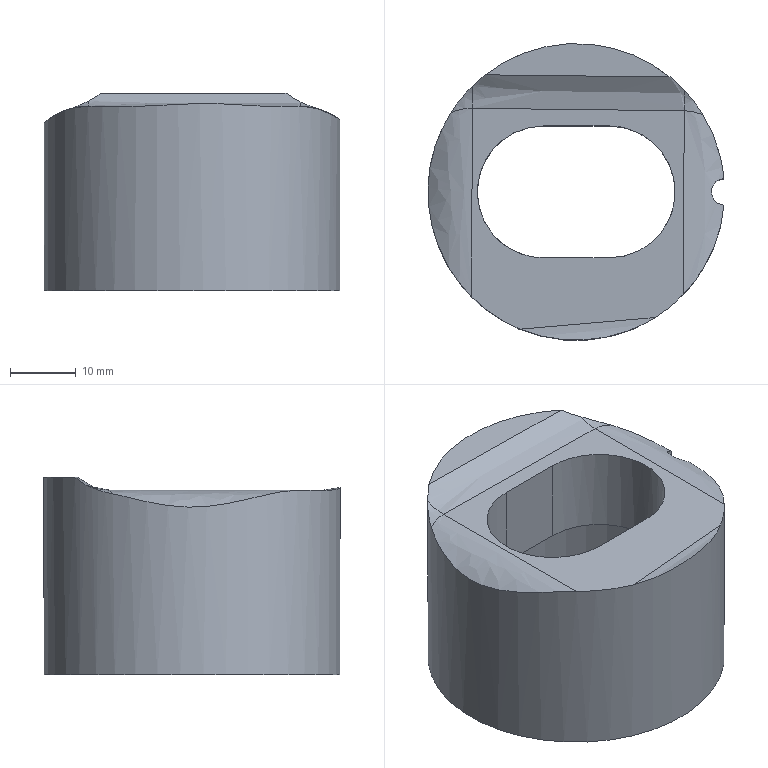Part | NX | features solid 2 | 1 solid | 17 faces | box 44.911 x 45 x 30 mm | volume 22561 mm3 | plane 6 | spline 6 | cylinder 5 | commonest cylinder face diameters 20 x2 4 x1 36 x1 45 x1
STEP:
#1=CARTESIAN_POINT('',(872.412,-199.998,17.));
#2=VERTEX_POINT('',#1);
#3=CARTESIAN_POINT('',(872.412,-199.998,42.909));
#4=VERTEX_POINT('',#3);
#5=CARTESIAN_POINT('',(872.412,-199.998,32.));
#6=DIRECTION('',(0.,0.,-1.));
#7=VECTOR('',#6,1000.);
#8=LINE('',#5,#7);
#9=EDGE_CURVE('',#2,#4,#8,.F.);
#10=ORIENTED_EDGE('',*,*,#9,.T.);
#11=CARTESIAN_POINT('',(866.197,-213.618,45.));
#12=VERTEX_POINT('',#11);
#13=CARTESIAN_POINT('',(872.412,-199.998,42.909));
#14=CARTESIAN_POINT('',(872.182,-202.576,43.073));
#15=CARTESIAN_POINT('',(870.861,-207.494,44.082));
#16=CARTESIAN_POINT('',(867.998,-211.75,45.));
#17=CARTESIAN_POINT('',(866.197,-213.618,45.));
#18=B_SPLINE_CURVE_WITH_KNOTS('',3,(#13,#14,#15,#16,#17),.UNSPECIFIED.,.F.,.F.,(4,1,4),(0.,0.007673,0.01535),.UNSPECIFIED.);
#19=EDGE_CURVE('',#4,#12,#18,.T.);
#20=ORIENTED_EDGE('',*,*,#19,.T.);
#21=CARTESIAN_POINT('',(861.953,-217.062,45.));
#22=VERTEX_POINT('',#21);
#23=CARTESIAN_POINT('',(850.,-198.,45.));
#24=DIRECTION('',(0.,0.,-1.));
#25=DIRECTION('',(-1.,0.,0.));
#26=AXIS2_PLACEMENT_3D('',#23,#24,#25);
#27=CIRCLE('',#26,22.5);
#28=EDGE_CURVE('',#22,#12,#27,.F.);
#29=ORIENTED_EDGE('',*,*,#28,.F.);
#30=CARTESIAN_POINT('',(841.476,-218.823,45.));
#31=VERTEX_POINT('',#30);
#32=CARTESIAN_POINT('',(841.477,-218.823,45.));
#33=CARTESIAN_POINT('',(843.14,-219.504,45.));
#34=CARTESIAN_POINT('',(846.561,-220.447,45.251));
#35=CARTESIAN_POINT('',(851.946,-220.631,45.502));
#36=CARTESIAN_POINT('',(857.214,-219.533,45.251));
#37=CARTESIAN_POINT('',(860.43,-218.017,45.));
#38=CARTESIAN_POINT('',(861.953,-217.063,45.));
#39=B_SPLINE_CURVE_WITH_KNOTS('',3,(#32,#33,#34,#35,#36,#37,#38),.UNSPECIFIED.,.F.,.F.,(4,1,1,1,4),(0.,0.00532,0.01064,0.01596,0.02128),.UNSPECIFIED.);
#40=EDGE_CURVE('',#31,#22,#39,.T.);
#41=ORIENTED_EDGE('',*,*,#40,.F.);
#42=CARTESIAN_POINT('',(834.154,-213.973,45.));
#43=VERTEX_POINT('',#42);
#44=CARTESIAN_POINT('',(850.,-198.,45.));
#45=DIRECTION('',(0.,0.,-1.));
#46=DIRECTION('',(-1.,0.,0.));
#47=AXIS2_PLACEMENT_3D('',#44,#45,#46);
#48=CIRCLE('',#47,22.5);
#49=EDGE_CURVE('',#43,#31,#48,.F.);
#50=ORIENTED_EDGE('',*,*,#49,.F.);
#51=CARTESIAN_POINT('',(831.005,-185.942,44.476));
#52=VERTEX_POINT('',#51);
#53=CARTESIAN_POINT('',(834.154,-213.973,45.));
#54=CARTESIAN_POINT('',(832.307,-212.14,45.));
#55=CARTESIAN_POINT('',(830.087,-208.98,44.262));
#56=CARTESIAN_POINT('',(828.298,-204.325,43.131));
#57=CARTESIAN_POINT('',(827.534,-200.55,42.483));
#58=CARTESIAN_POINT('',(827.428,-196.687,42.375));
#59=CARTESIAN_POINT('',(828.171,-191.587,43.034));
#60=CARTESIAN_POINT('',(829.64,-188.092,44.017));
#61=CARTESIAN_POINT('',(831.001,-185.947,44.475));
#62=B_SPLINE_CURVE_WITH_KNOTS('',3,(#53,#54,#55,#56,#57,#58,#59,#60,#61),.UNSPECIFIED.,.F.,.F.,(4,1,1,1,1,1,4),(0.,0.007693,0.01154,0.01539,0.01923,0.02308,0.03077),.UNSPECIFIED.);
#63=EDGE_CURVE('',#43,#52,#62,.T.);
#64=ORIENTED_EDGE('',*,*,#63,.T.);
#65=CARTESIAN_POINT('',(834.237,-181.945,45.803));
#66=VERTEX_POINT('',#65);
#67=CARTESIAN_POINT('',(834.237,-181.945,45.803));
#68=CARTESIAN_POINT('',(833.043,-183.117,45.205));
#69=CARTESIAN_POINT('',(831.945,-184.461,44.793));
#70=CARTESIAN_POINT('',(831.008,-185.936,44.477));
#71=B_SPLINE_CURVE_WITH_KNOTS('',3,(#67,#68,#69,#70),.UNSPECIFIED.,.F.,.F.,(4,4),(0.,0.005314),.UNSPECIFIED.);
#72=EDGE_CURVE('',#66,#52,#71,.T.);
#73=ORIENTED_EDGE('',*,*,#72,.F.);
#74=CARTESIAN_POINT('',(836.183,-180.242,47.));
#75=VERTEX_POINT('',#74);
#76=CARTESIAN_POINT('',(836.183,-180.242,47.));
#77=CARTESIAN_POINT('',(835.53,-180.75,46.523));
#78=CARTESIAN_POINT('',(834.879,-181.315,46.124));
#79=CARTESIAN_POINT('',(834.237,-181.945,45.803));
#80=B_SPLINE_CURVE_WITH_KNOTS('',3,(#76,#77,#78,#79),.UNSPECIFIED.,.F.,.F.,(4,4),(0.,0.002849),.UNSPECIFIED.);
#81=EDGE_CURVE('',#75,#66,#80,.T.);
#82=ORIENTED_EDGE('',*,*,#81,.F.);
#83=CARTESIAN_POINT('',(864.222,-180.565,47.));
#84=VERTEX_POINT('',#83);
#85=CARTESIAN_POINT('',(850.,-198.,47.));
#86=DIRECTION('',(0.,0.,-1.));
#87=DIRECTION('',(-1.,0.,0.));
#88=AXIS2_PLACEMENT_3D('',#85,#86,#87);
#89=CIRCLE('',#88,22.5);
#90=EDGE_CURVE('',#75,#84,#89,.T.);
#91=ORIENTED_EDGE('',*,*,#90,.T.);
#92=CARTESIAN_POINT('',(866.428,-182.626,45.655));
#93=VERTEX_POINT('',#92);
#94=CARTESIAN_POINT('',(866.428,-182.626,45.655));
#95=CARTESIAN_POINT('',(865.707,-181.854,45.996));
#96=CARTESIAN_POINT('',(864.967,-181.172,46.445));
#97=CARTESIAN_POINT('',(864.222,-180.565,47.));
#98=B_SPLINE_CURVE_WITH_KNOTS('',3,(#94,#95,#96,#97),.UNSPECIFIED.,.F.,.F.,(4,4),(0.,0.003305),.UNSPECIFIED.);
#99=EDGE_CURVE('',#93,#84,#98,.T.);
#100=ORIENTED_EDGE('',*,*,#99,.F.);
#101=CARTESIAN_POINT('',(869.203,-186.274,44.595));
#102=VERTEX_POINT('',#101);
#103=CARTESIAN_POINT('',(869.203,-186.274,44.595));
#104=CARTESIAN_POINT('',(868.389,-184.941,44.837));
#105=CARTESIAN_POINT('',(867.457,-183.724,45.169));
#106=CARTESIAN_POINT('',(866.428,-182.626,45.655));
#107=B_SPLINE_CURVE_WITH_KNOTS('',3,(#103,#104,#105,#106),.UNSPECIFIED.,.F.,.F.,(4,4),(0.,0.004705),.UNSPECIFIED.);
#108=EDGE_CURVE('',#102,#93,#107,.T.);
#109=ORIENTED_EDGE('',*,*,#108,.F.);
#110=CARTESIAN_POINT('',(872.412,-196.002,42.93));
#111=VERTEX_POINT('',#110);
#112=CARTESIAN_POINT('',(869.204,-186.275,44.595));
#113=CARTESIAN_POINT('',(871.004,-189.224,44.06));
#114=CARTESIAN_POINT('',(872.1,-192.509,43.188));
#115=CARTESIAN_POINT('',(872.412,-196.002,42.93));
#116=B_SPLINE_CURVE_WITH_KNOTS('',3,(#112,#113,#114,#115),.UNSPECIFIED.,.F.,.F.,(4,4),(0.0008951,0.0113),.UNSPECIFIED.);
#117=EDGE_CURVE('',#102,#111,#116,.T.);
#118=ORIENTED_EDGE('',*,*,#117,.T.);
#119=CARTESIAN_POINT('',(872.412,-196.002,17.));
#120=VERTEX_POINT('',#119);
#121=CARTESIAN_POINT('',(872.412,-196.002,32.));
#122=DIRECTION('',(0.,0.,-1.));
#123=VECTOR('',#122,1000.);
#124=LINE('',#121,#123);
#125=EDGE_CURVE('',#111,#120,#124,.T.);
#126=ORIENTED_EDGE('',*,*,#125,.T.);
#127=CARTESIAN_POINT('',(850.,-198.,17.));
#128=DIRECTION('',(0.,0.,-1.));
#129=DIRECTION('',(-1.,0.,0.));
#130=AXIS2_PLACEMENT_3D('',#127,#128,#129);
#131=CIRCLE('',#130,22.5);
#132=EDGE_CURVE('',#2,#120,#131,.T.);
#133=ORIENTED_EDGE('',*,*,#132,.F.);
#134=EDGE_LOOP('',(#10,#20,#29,#41,#50,#64,#73,#82,#91,#100,#109,#118,#126,#133));
#135=FACE_BOUND('',#134,.T.);
#136=CARTESIAN_POINT('',(850.,-198.,17.));
#137=DIRECTION('',(0.,0.,1.));
#138=DIRECTION('',(-1.,0.,0.));
#139=AXIS2_PLACEMENT_3D('',#136,#137,#138);
#140=CYLINDRICAL_SURFACE('',#139,22.5);
#141=ADVANCED_FACE('',(#135),#140,.T.);
#142=CARTESIAN_POINT('',(845.,-208.,32.));
#143=VERTEX_POINT('',#142);
#144=CARTESIAN_POINT('',(845.,-208.,45.));
#145=VERTEX_POINT('',#144);
#146=CARTESIAN_POINT('',(845.,-208.,-233.));
#147=DIRECTION('',(0.,0.,1.));
#148=VECTOR('',#147,1000.);
#149=LINE('',#146,#148);
#150=EDGE_CURVE('',#143,#145,#149,.T.);
#151=ORIENTED_EDGE('',*,*,#150,.T.);
#152=CARTESIAN_POINT('',(855.,-208.,45.));
#153=VERTEX_POINT('',#152);
#154=CARTESIAN_POINT('',(845.,-208.,45.));
#155=CARTESIAN_POINT('',(848.334,-208.,45.));
#156=CARTESIAN_POINT('',(851.667,-208.,45.));
#157=CARTESIAN_POINT('',(855.,-208.,45.));
#158=B_SPLINE_CURVE_WITH_KNOTS('',3,(#154,#155,#156,#157),.UNSPECIFIED.,.F.,.F.,(4,4),(0.,1.),.UNSPECIFIED.);
#159=EDGE_CURVE('',#145,#153,#158,.T.);
#160=ORIENTED_EDGE('',*,*,#159,.T.);
#161=CARTESIAN_POINT('',(855.,-208.,32.));
#162=VERTEX_POINT('',#161);
#163=CARTESIAN_POINT('',(855.,-208.,-233.));
#164=DIRECTION('',(0.,0.,1.));
#165=VECTOR('',#164,1000.);
#166=LINE('',#163,#165);
#167=EDGE_CURVE('',#162,#153,#166,.T.);
#168=ORIENTED_EDGE('',*,*,#167,.F.);
#169=CARTESIAN_POINT('',(845.,-208.,32.));
#170=DIRECTION('',(-1.,0.,0.));
#171=VECTOR('',#170,1000.);
#172=LINE('',#169,#171);
#173=EDGE_CURVE('',#162,#143,#172,.T.);
#174=ORIENTED_EDGE('',*,*,#173,.T.);
#175=EDGE_LOOP('',(#151,#160,#168,#174));
#176=FACE_BOUND('',#175,.T.);
#177=CARTESIAN_POINT('',(845.,-208.,-233.));
#178=DIRECTION('',(0.,1.,0.));
#179=DIRECTION('',(0.,0.,1.));
#180=AXIS2_PLACEMENT_3D('',#177,#178,#179);
#181=PLANE('',#180);
#182=ADVANCED_FACE('',(#176),#181,.T.);
#183=CARTESIAN_POINT('',(855.,-188.,45.));
#184=VERTEX_POINT('',#183);
#185=CARTESIAN_POINT('',(855.,-208.,45.));
#186=CARTESIAN_POINT('',(855.109,-207.999,45.));
#187=CARTESIAN_POINT('',(855.233,-207.998,45.));
#188=CARTESIAN_POINT('',(855.579,-207.987,45.));
#189=CARTESIAN_POINT('',(856.138,-207.945,45.));
#190=CARTESIAN_POINT('',(856.956,-207.826,45.));
#191=CARTESIAN_POINT('',(857.897,-207.589,45.));
#192=CARTESIAN_POINT('',(859.141,-207.143,45.));
#193=CARTESIAN_POINT('',(860.59,-206.373,45.));
#194=CARTESIAN_POINT('',(862.623,-204.701,45.));
#195=CARTESIAN_POINT('',(864.48,-201.929,45.));
#196=CARTESIAN_POINT('',(865.261,-198.,45.));
#197=CARTESIAN_POINT('',(864.48,-194.072,45.));
#198=CARTESIAN_POINT('',(862.623,-191.299,45.));
#199=CARTESIAN_POINT('',(860.591,-189.628,45.));
#200=CARTESIAN_POINT('',(859.141,-188.857,45.));
#201=CARTESIAN_POINT('',(857.898,-188.411,45.));
#202=CARTESIAN_POINT('',(856.956,-188.174,45.));
#203=CARTESIAN_POINT('',(856.138,-188.055,45.));
#204=CARTESIAN_POINT('',(855.579,-188.013,45.));
#205=CARTESIAN_POINT('',(855.233,-188.004,45.));
#206=CARTESIAN_POINT('',(855.11,-188.002,45.));
#207=CARTESIAN_POINT('',(855.,-188.,45.));
#208=B_SPLINE_CURVE_WITH_KNOTS('',3,(#185,#186,#187,#188,#189,#190,#191,#192,#193,#194,#195,#196,#197,#198,#199,#200,#201,#202,#203,#204,#205,#206,#207),.UNSPECIFIED.,.F.,.F.,(4,1,1,1,1,1,1,1,1,1,1,1,1,1,1,1,1,1,1,1,4),(0.,0.007813,0.01563,0.03125,0.0625,0.09375,0.125,0.1875,0.25,0.375,0.5,0.625,0.75,0.8125,0.875,0.9063,0.9375,0.9688,0.9844,0.9922,1.),.UNSPECIFIED.);
#209=EDGE_CURVE('',#184,#153,#208,.F.);
#210=ORIENTED_EDGE('',*,*,#209,.F.);
#211=CARTESIAN_POINT('',(855.,-188.,32.));
#212=VERTEX_POINT('',#211);
#213=CARTESIAN_POINT('',(855.,-188.,-233.));
#214=DIRECTION('',(0.,0.,1.));
#215=VECTOR('',#214,1000.);
#216=LINE('',#213,#215);
#217=EDGE_CURVE('',#212,#184,#216,.T.);
#218=ORIENTED_EDGE('',*,*,#217,.F.);
#219=CARTESIAN_POINT('',(855.,-198.,32.));
#220=DIRECTION('',(0.,0.,-1.));
#221=DIRECTION('',(-1.,0.,0.));
#222=AXIS2_PLACEMENT_3D('',#219,#220,#221);
#223=CIRCLE('',#222,10.);
#224=EDGE_CURVE('',#162,#212,#223,.F.);
#225=ORIENTED_EDGE('',*,*,#224,.F.);
#226=ORIENTED_EDGE('',*,*,#167,.T.);
#227=EDGE_LOOP('',(#210,#218,#225,#226));
#228=FACE_BOUND('',#227,.T.);
#229=CARTESIAN_POINT('',(855.,-198.,-233.));
#230=DIRECTION('',(0.,0.,1.));
#231=DIRECTION('',(-1.,0.,0.));
#232=AXIS2_PLACEMENT_3D('',#229,#230,#231);
#233=CYLINDRICAL_SURFACE('',#232,10.);
#234=ADVANCED_FACE('',(#228),#233,.F.);
#235=CARTESIAN_POINT('',(845.,-188.,45.));
#236=VERTEX_POINT('',#235);
#237=CARTESIAN_POINT('',(845.,-188.,45.));
#238=CARTESIAN_POINT('',(848.334,-188.,45.));
#239=CARTESIAN_POINT('',(851.667,-188.,45.));
#240=CARTESIAN_POINT('',(855.,-188.,45.));
#241=B_SPLINE_CURVE_WITH_KNOTS('',3,(#237,#238,#239,#240),.UNSPECIFIED.,.F.,.F.,(4,4),(0.,1.),.UNSPECIFIED.);
#242=EDGE_CURVE('',#236,#184,#241,.T.);
#243=ORIENTED_EDGE('',*,*,#242,.F.);
#244=CARTESIAN_POINT('',(845.,-188.,32.));
#245=VERTEX_POINT('',#244);
#246=CARTESIAN_POINT('',(845.,-188.,-233.));
#247=DIRECTION('',(0.,0.,1.));
#248=VECTOR('',#247,1000.);
#249=LINE('',#246,#248);
#250=EDGE_CURVE('',#245,#236,#249,.T.);
#251=ORIENTED_EDGE('',*,*,#250,.F.);
#252=CARTESIAN_POINT('',(845.,-188.,32.));
#253=DIRECTION('',(-1.,0.,0.));
#254=VECTOR('',#253,1000.);
#255=LINE('',#252,#254);
#256=EDGE_CURVE('',#212,#245,#255,.T.);
#257=ORIENTED_EDGE('',*,*,#256,.F.);
#258=ORIENTED_EDGE('',*,*,#217,.T.);
#259=EDGE_LOOP('',(#243,#251,#257,#258));
#260=FACE_BOUND('',#259,.T.);
#261=CARTESIAN_POINT('',(845.,-188.,-233.));
#262=DIRECTION('',(0.,1.,0.));
#263=DIRECTION('',(0.,0.,1.));
#264=AXIS2_PLACEMENT_3D('',#261,#262,#263);
#265=PLANE('',#264);
#266=ADVANCED_FACE('',(#260),#265,.F.);
#267=CARTESIAN_POINT('',(845.,-188.,45.));
#268=CARTESIAN_POINT('',(844.891,-188.001,45.));
#269=CARTESIAN_POINT('',(844.767,-188.002,45.));
#270=CARTESIAN_POINT('',(844.421,-188.013,45.));
#271=CARTESIAN_POINT('',(843.863,-188.055,45.));
#272=CARTESIAN_POINT('',(843.044,-188.174,45.));
#273=CARTESIAN_POINT('',(842.103,-188.411,45.));
#274=CARTESIAN_POINT('',(840.859,-188.857,45.));
#275=CARTESIAN_POINT('',(839.41,-189.627,45.));
#276=CARTESIAN_POINT('',(837.377,-191.299,45.));
#277=CARTESIAN_POINT('',(835.521,-194.071,45.));
#278=CARTESIAN_POINT('',(834.74,-198.,45.));
#279=CARTESIAN_POINT('',(835.52,-201.928,45.));
#280=CARTESIAN_POINT('',(837.378,-204.701,45.));
#281=CARTESIAN_POINT('',(839.409,-206.372,45.));
#282=CARTESIAN_POINT('',(840.86,-207.143,45.));
#283=CARTESIAN_POINT('',(842.102,-207.589,45.));
#284=CARTESIAN_POINT('',(843.044,-207.826,45.));
#285=CARTESIAN_POINT('',(843.863,-207.945,45.));
#286=CARTESIAN_POINT('',(844.421,-207.987,45.));
#287=CARTESIAN_POINT('',(844.767,-207.996,45.));
#288=CARTESIAN_POINT('',(844.891,-207.998,45.));
#289=CARTESIAN_POINT('',(845.,-208.,45.));
#290=B_SPLINE_CURVE_WITH_KNOTS('',3,(#267,#268,#269,#270,#271,#272,#273,#274,#275,#276,#277,#278,#279,#280,#281,#282,#283,#284,#285,#286,#287,#288,#289),.UNSPECIFIED.,.F.,.F.,(4,1,1,1,1,1,1,1,1,1,1,1,1,1,1,1,1,1,1,1,4),(0.,0.007812,0.01562,0.03125,0.0625,0.09375,0.125,0.1875,0.25,0.375,0.5,0.625,0.75,0.8125,0.875,0.9062,0.9375,0.9688,0.9844,0.9922,1.),.UNSPECIFIED.);
#291=EDGE_CURVE('',#145,#236,#290,.F.);
#292=ORIENTED_EDGE('',*,*,#291,.F.);
#293=ORIENTED_EDGE('',*,*,#150,.F.);
#294=CARTESIAN_POINT('',(845.,-198.,32.));
#295=DIRECTION('',(0.,0.,-1.));
#296=DIRECTION('',(-1.,0.,0.));
#297=AXIS2_PLACEMENT_3D('',#294,#295,#296);
#298=CIRCLE('',#297,10.);
#299=EDGE_CURVE('',#245,#143,#298,.F.);
#300=ORIENTED_EDGE('',*,*,#299,.F.);
#301=ORIENTED_EDGE('',*,*,#250,.T.);
#302=EDGE_LOOP('',(#292,#293,#300,#301));
#303=FACE_BOUND('',#302,.T.);
#304=CARTESIAN_POINT('',(845.,-198.,-233.));
#305=DIRECTION('',(0.,0.,1.));
#306=DIRECTION('',(-1.,0.,0.));
#307=AXIS2_PLACEMENT_3D('',#304,#305,#306);
#308=CYLINDRICAL_SURFACE('',#307,10.);
#309=ADVANCED_FACE('',(#303),#308,.F.);
#310=CARTESIAN_POINT('',(872.412,-199.998,42.909));
#311=CARTESIAN_POINT('',(871.971,-199.978,43.25));
#312=CARTESIAN_POINT('',(871.024,-199.646,43.845));
#313=CARTESIAN_POINT('',(870.243,-198.012,44.189));
#314=CARTESIAN_POINT('',(871.006,-196.364,43.865));
#315=CARTESIAN_POINT('',(871.968,-196.022,43.271));
#316=CARTESIAN_POINT('',(872.412,-196.002,42.93));
#317=B_SPLINE_CURVE_WITH_KNOTS('',3,(#310,#311,#312,#313,#314,#315,#316),.UNSPECIFIED.,.F.,.F.,(4,1,1,1,4),(0.,0.001645,0.00329,0.004935,0.00658),.UNSPECIFIED.);
#318=EDGE_CURVE('',#4,#111,#317,.T.);
#319=ORIENTED_EDGE('',*,*,#318,.F.);
#320=ORIENTED_EDGE('',*,*,#9,.F.);
#321=CARTESIAN_POINT('',(872.5,-198.,17.));
#322=DIRECTION('',(0.,0.,-1.));
#323=DIRECTION('',(-1.,0.,0.));
#324=AXIS2_PLACEMENT_3D('',#321,#322,#323);
#325=CIRCLE('',#324,2.);
#326=EDGE_CURVE('',#2,#120,#325,.T.);
#327=ORIENTED_EDGE('',*,*,#326,.T.);
#328=ORIENTED_EDGE('',*,*,#125,.F.);
#329=EDGE_LOOP('',(#319,#320,#327,#328));
#330=FACE_BOUND('',#329,.T.);
#331=CARTESIAN_POINT('',(872.5,-198.,47.));
#332=DIRECTION('',(0.,0.,-1.));
#333=DIRECTION('',(1.,0.,0.));
#334=AXIS2_PLACEMENT_3D('',#331,#332,#333);
#335=CYLINDRICAL_SURFACE('',#334,2.);
#336=ADVANCED_FACE('',(#330),#335,.F.);
#337=ORIENTED_EDGE('',*,*,#132,.T.);
#338=ORIENTED_EDGE('',*,*,#326,.F.);
#339=EDGE_LOOP('',(#337,#338));
#340=FACE_BOUND('',#339,.T.);
#341=CARTESIAN_POINT('',(832.,-198.,17.));
#342=VERTEX_POINT('',#341);
#343=CARTESIAN_POINT('',(850.,-198.,17.));
#344=DIRECTION('',(0.,0.,-1.));
#345=DIRECTION('',(-1.,0.,0.));
#346=AXIS2_PLACEMENT_3D('',#343,#344,#345);
#347=CIRCLE('',#346,18.);
#348=EDGE_CURVE('',#342,#342,#347,.F.);
#349=ORIENTED_EDGE('',*,*,#348,.T.);
#350=EDGE_LOOP('',(#349));
#351=FACE_BOUND('',#350,.T.);
#352=CARTESIAN_POINT('',(850.,-198.,17.));
#353=DIRECTION('',(0.,0.,1.));
#354=DIRECTION('',(-1.,0.,0.));
#355=AXIS2_PLACEMENT_3D('',#352,#353,#354);
#356=PLANE('',#355);
#357=ADVANCED_FACE('',(#340,#351),#356,.F.);
#358=CARTESIAN_POINT('',(864.222,-180.565,47.));
#359=CARTESIAN_POINT('',(854.876,-180.451,47.));
#360=CARTESIAN_POINT('',(845.53,-180.344,47.));
#361=CARTESIAN_POINT('',(836.183,-180.242,47.));
#362=B_SPLINE_CURVE_WITH_KNOTS('',3,(#358,#359,#360,#361),.UNSPECIFIED.,.F.,.F.,(4,4),(0.002231,0.03027),.UNSPECIFIED.);
#363=EDGE_CURVE('',#84,#75,#362,.T.);
#364=ORIENTED_EDGE('',*,*,#363,.F.);
#365=ORIENTED_EDGE('',*,*,#90,.F.);
#366=EDGE_LOOP('',(#364,#365));
#367=FACE_BOUND('',#366,.T.);
#368=CARTESIAN_POINT('',(850.,-198.,47.));
#369=DIRECTION('',(0.,0.,1.));
#370=DIRECTION('',(-1.,0.,0.));
#371=AXIS2_PLACEMENT_3D('',#368,#369,#370);
#372=PLANE('',#371);
#373=ADVANCED_FACE('',(#367),#372,.T.);
#374=CARTESIAN_POINT('',(832.,-198.,32.));
#375=VERTEX_POINT('',#374);
#376=CARTESIAN_POINT('',(850.,-198.,32.));
#377=DIRECTION('',(0.,0.,-1.));
#378=DIRECTION('',(-1.,0.,0.));
#379=AXIS2_PLACEMENT_3D('',#376,#377,#378);
#380=CIRCLE('',#379,18.);
#381=EDGE_CURVE('',#375,#375,#380,.T.);
#382=ORIENTED_EDGE('',*,*,#381,.F.);
#383=EDGE_LOOP('',(#382));
#384=FACE_BOUND('',#383,.T.);
#385=ORIENTED_EDGE('',*,*,#348,.F.);
#386=EDGE_LOOP('',(#385));
#387=FACE_BOUND('',#386,.T.);
#388=CARTESIAN_POINT('',(850.,-198.,39.));
#389=DIRECTION('',(0.,0.,-1.));
#390=DIRECTION('',(1.,0.,0.));
#391=AXIS2_PLACEMENT_3D('',#388,#389,#390);
#392=CYLINDRICAL_SURFACE('',#391,18.);
#393=ADVANCED_FACE('',(#384,#387),#392,.F.);
#394=ORIENTED_EDGE('',*,*,#173,.F.);
#395=ORIENTED_EDGE('',*,*,#224,.T.);
#396=ORIENTED_EDGE('',*,*,#256,.T.);
#397=ORIENTED_EDGE('',*,*,#299,.T.);
#398=EDGE_LOOP('',(#394,#395,#396,#397));
#399=FACE_BOUND('',#398,.T.);
#400=ORIENTED_EDGE('',*,*,#381,.T.);
#401=EDGE_LOOP('',(#400));
#402=FACE_BOUND('',#401,.T.);
#403=CARTESIAN_POINT('',(850.,-198.,32.));
#404=DIRECTION('',(0.,0.,1.));
#405=DIRECTION('',(-1.,0.,0.));
#406=AXIS2_PLACEMENT_3D('',#403,#404,#405);
#407=PLANE('',#406);
#408=ADVANCED_FACE('',(#399,#402),#407,.F.);
#409=ORIENTED_EDGE('',*,*,#108,.T.);
#410=CARTESIAN_POINT('',(866.391,-185.691,45.));
#411=VERTEX_POINT('',#410);
#412=CARTESIAN_POINT('',(866.391,-185.691,45.));
#413=CARTESIAN_POINT('',(866.403,-184.672,45.));
#414=CARTESIAN_POINT('',(866.416,-183.603,45.217));
#415=CARTESIAN_POINT('',(866.428,-182.626,45.655));
#416=B_SPLINE_CURVE_WITH_KNOTS('',3,(#412,#413,#414,#415),.UNSPECIFIED.,.F.,.F.,(4,4),(0.,0.4737),.UNSPECIFIED.);
#417=EDGE_CURVE('',#93,#411,#416,.F.);
#418=ORIENTED_EDGE('',*,*,#417,.T.);
#419=CARTESIAN_POINT('',(869.204,-186.274,44.595));
#420=CARTESIAN_POINT('',(868.307,-185.933,44.859));
#421=CARTESIAN_POINT('',(867.345,-185.706,45.));
#422=CARTESIAN_POINT('',(866.391,-185.691,45.));
#423=B_SPLINE_CURVE_WITH_KNOTS('',3,(#419,#420,#421,#422),.UNSPECIFIED.,.F.,.F.,(4,4),(0.626,1.),.UNSPECIFIED.);
#424=EDGE_CURVE('',#102,#411,#423,.T.);
#425=ORIENTED_EDGE('',*,*,#424,.F.);
#426=EDGE_LOOP('',(#409,#418,#425));
#427=FACE_BOUND('',#426,.T.);
#428=CARTESIAN_POINT('',(869.22,-186.28,44.59));
#429=CARTESIAN_POINT('',(869.575,-184.525,44.489));
#430=CARTESIAN_POINT('',(870.125,-182.962,45.177));
#431=CARTESIAN_POINT('',(868.918,-186.165,44.68));
#432=CARTESIAN_POINT('',(869.245,-184.44,44.599));
#433=CARTESIAN_POINT('',(869.736,-182.897,45.281));
#434=CARTESIAN_POINT('',(868.61,-186.061,44.755));
#435=CARTESIAN_POINT('',(868.905,-184.363,44.692));
#436=CARTESIAN_POINT('',(869.338,-182.837,45.37));
#437=CARTESIAN_POINT('',(867.987,-185.889,44.877));
#438=CARTESIAN_POINT('',(868.212,-184.234,44.843));
#439=CARTESIAN_POINT('',(868.527,-182.735,45.514));
#440=CARTESIAN_POINT('',(867.672,-185.82,44.923));
#441=CARTESIAN_POINT('',(867.858,-184.181,44.902));
#442=CARTESIAN_POINT('',(868.114,-182.693,45.569));
#443=CARTESIAN_POINT('',(867.03,-185.723,44.985));
#444=CARTESIAN_POINT('',(867.134,-184.105,44.98));
#445=CARTESIAN_POINT('',(867.27,-182.632,45.644));
#446=CARTESIAN_POINT('',(866.71,-185.696,45.));
#447=CARTESIAN_POINT('',(866.771,-184.084,45.));
#448=CARTESIAN_POINT('',(866.848,-182.614,45.663));
#449=CARTESIAN_POINT('',(866.391,-185.691,45.));
#450=CARTESIAN_POINT('',(866.411,-184.078,45.));
#451=CARTESIAN_POINT('',(866.429,-182.608,45.663));
#452=(BOUNDED_SURFACE()B_SPLINE_SURFACE(3,2,((#428,#429,#430),(#431,#432,#433),(#434,#435,#436),(#437,#438,#439),(#440,#441,#442),(#443,#444,#445),(#446,#447,#448),(#449,#450,#451)),.UNSPECIFIED.,.F.,.F.,.F.)B_SPLINE_SURFACE_WITH_KNOTS((4,2,2,4),(3,3),(0.6238,0.75,0.875,1.),(0.,0.4765),.UNSPECIFIED.)GEOMETRIC_REPRESENTATION_ITEM()RATIONAL_B_SPLINE_SURFACE(((1.,0.9432,0.9405),(1.,0.9454,0.9429),(1.,0.9473,0.9448),(1.,0.9504,0.9481),(1.,0.9516,0.9493),(1.,0.9532,0.951),(1.,0.9536,0.9514),(1.,0.9536,0.9514)))REPRESENTATION_ITEM('')SURFACE());
#453=ADVANCED_FACE('',(#427),#452,.F.);
#454=ORIENTED_EDGE('',*,*,#81,.T.);
#455=CARTESIAN_POINT('',(834.201,-185.32,45.));
#456=VERTEX_POINT('',#455);
#457=CARTESIAN_POINT('',(834.201,-185.32,45.));
#458=CARTESIAN_POINT('',(834.213,-184.192,45.));
#459=CARTESIAN_POINT('',(834.226,-183.004,45.269));
#460=CARTESIAN_POINT('',(834.237,-181.945,45.803));
#461=B_SPLINE_CURVE_WITH_KNOTS('',3,(#457,#458,#459,#460),.UNSPECIFIED.,.F.,.F.,(4,4),(0.,0.5243),.UNSPECIFIED.);
#462=EDGE_CURVE('',#66,#456,#461,.F.);
#463=ORIENTED_EDGE('',*,*,#462,.T.);
#464=CARTESIAN_POINT('',(834.201,-185.32,45.));
#465=CARTESIAN_POINT('',(844.931,-185.444,45.));
#466=CARTESIAN_POINT('',(855.661,-185.567,45.));
#467=CARTESIAN_POINT('',(866.391,-185.691,45.));
#468=B_SPLINE_CURVE_WITH_KNOTS('',3,(#464,#465,#466,#467),.UNSPECIFIED.,.F.,.F.,(4,4),(0.,1.),.UNSPECIFIED.);
#469=EDGE_CURVE('',#456,#411,#468,.T.);
#470=ORIENTED_EDGE('',*,*,#469,.T.);
#471=ORIENTED_EDGE('',*,*,#417,.F.);
#472=ORIENTED_EDGE('',*,*,#99,.T.);
#473=ORIENTED_EDGE('',*,*,#363,.T.);
#474=EDGE_LOOP('',(#454,#463,#470,#471,#472,#473));
#475=FACE_BOUND('',#474,.T.);
#476=CARTESIAN_POINT('',(866.391,-185.691,45.));
#477=CARTESIAN_POINT('',(866.427,-182.749,45.));
#478=CARTESIAN_POINT('',(866.453,-180.592,47.));
#479=CARTESIAN_POINT('',(855.661,-185.559,45.));
#480=CARTESIAN_POINT('',(855.695,-182.617,45.));
#481=CARTESIAN_POINT('',(855.72,-180.46,47.));
#482=CARTESIAN_POINT('',(844.931,-185.436,45.));
#483=CARTESIAN_POINT('',(844.964,-182.495,45.));
#484=CARTESIAN_POINT('',(844.988,-180.338,47.));
#485=CARTESIAN_POINT('',(834.201,-185.32,45.));
#486=CARTESIAN_POINT('',(834.232,-182.379,45.));
#487=CARTESIAN_POINT('',(834.256,-180.221,47.));
#488=(BOUNDED_SURFACE()B_SPLINE_SURFACE(3,2,((#476,#477,#478),(#479,#480,#481),(#482,#483,#484),(#485,#486,#487)),.UNSPECIFIED.,.F.,.F.,.F.)B_SPLINE_SURFACE_WITH_KNOTS((4,4),(3,3),(0.,1.),(0.,0.8372),.PIECEWISE_BEZIER_KNOTS.)GEOMETRIC_REPRESENTATION_ITEM()RATIONAL_B_SPLINE_SURFACE(((1.,0.9185,0.9735),(1.,0.9185,0.9735),(1.,0.9185,0.9735),(1.,0.9185,0.9735)))REPRESENTATION_ITEM('')SURFACE());
#489=ADVANCED_FACE('',(#475),#488,.F.);
#490=ORIENTED_EDGE('',*,*,#72,.T.);
#491=CARTESIAN_POINT('',(834.201,-185.32,45.));
#492=CARTESIAN_POINT('',(833.097,-185.301,45.));
#493=CARTESIAN_POINT('',(832.024,-185.555,44.819));
#494=CARTESIAN_POINT('',(831.006,-185.945,44.476));
#495=B_SPLINE_CURVE_WITH_KNOTS('',3,(#491,#492,#493,#494),.UNSPECIFIED.,.F.,.F.,(4,4),(0.,0.4046),.UNSPECIFIED.);
#496=EDGE_CURVE('',#456,#52,#495,.T.);
#497=ORIENTED_EDGE('',*,*,#496,.F.);
#498=ORIENTED_EDGE('',*,*,#462,.F.);
#499=EDGE_LOOP('',(#490,#497,#498));
#500=FACE_BOUND('',#499,.T.);
#501=CARTESIAN_POINT('',(834.201,-185.32,45.));
#502=CARTESIAN_POINT('',(834.22,-183.526,45.));
#503=CARTESIAN_POINT('',(834.237,-181.926,45.812));
#504=CARTESIAN_POINT('',(833.86,-185.314,45.));
#505=CARTESIAN_POINT('',(833.829,-183.52,45.001));
#506=CARTESIAN_POINT('',(833.775,-181.92,45.813));
#507=CARTESIAN_POINT('',(833.522,-185.333,44.983));
#508=CARTESIAN_POINT('',(833.443,-183.532,44.979));
#509=CARTESIAN_POINT('',(833.317,-181.927,45.792));
#510=CARTESIAN_POINT('',(832.856,-185.416,44.915));
#511=CARTESIAN_POINT('',(832.683,-183.588,44.893));
#512=CARTESIAN_POINT('',(832.416,-181.966,45.713));
#513=CARTESIAN_POINT('',(832.526,-185.48,44.864));
#514=CARTESIAN_POINT('',(832.308,-183.632,44.828));
#515=CARTESIAN_POINT('',(831.971,-181.998,45.654));
#516=CARTESIAN_POINT('',(832.036,-185.604,44.765));
#517=CARTESIAN_POINT('',(831.757,-183.716,44.702));
#518=CARTESIAN_POINT('',(831.315,-182.058,45.539));
#519=CARTESIAN_POINT('',(831.874,-185.649,44.727));
#520=CARTESIAN_POINT('',(831.575,-183.747,44.655));
#521=CARTESIAN_POINT('',(831.098,-182.08,45.495));
#522=CARTESIAN_POINT('',(831.551,-185.75,44.644));
#523=CARTESIAN_POINT('',(831.215,-183.815,44.552));
#524=CARTESIAN_POINT('',(830.668,-182.129,45.4));
#525=CARTESIAN_POINT('',(831.39,-185.804,44.599));
#526=CARTESIAN_POINT('',(831.037,-183.852,44.495));
#527=CARTESIAN_POINT('',(830.454,-182.155,45.348));
#528=CARTESIAN_POINT('',(831.149,-185.891,44.524));
#529=CARTESIAN_POINT('',(830.772,-183.91,44.402));
#530=CARTESIAN_POINT('',(830.136,-182.196,45.263));
#531=CARTESIAN_POINT('',(831.068,-185.921,44.497));
#532=CARTESIAN_POINT('',(830.683,-183.93,44.37));
#533=CARTESIAN_POINT('',(830.029,-182.21,45.233));
#534=CARTESIAN_POINT('',(830.987,-185.952,44.47));
#535=CARTESIAN_POINT('',(830.595,-183.95,44.336));
#536=CARTESIAN_POINT('',(829.923,-182.225,45.203));
#537=(BOUNDED_SURFACE()B_SPLINE_SURFACE(3,2,((#501,#502,#503),(#504,#505,#506),(#507,#508,#509),(#510,#511,#512),(#513,#514,#515),(#516,#517,#518),(#519,#520,#521),(#522,#523,#524),(#525,#526,#527),(#528,#529,#530),(#531,#532,#533),(#534,#535,#536)),.UNSPECIFIED.,.F.,.F.,.F.)B_SPLINE_SURFACE_WITH_KNOTS((4,2,2,2,2,4),(3,3),(0.,0.125,0.25,0.3125,0.375,0.407),(0.,0.5274),.UNSPECIFIED.)GEOMETRIC_REPRESENTATION_ITEM()RATIONAL_B_SPLINE_SURFACE(((1.,0.9487,0.9515),(1.,0.9487,0.9515),(1.,0.9482,0.9511),(1.,0.9464,0.9494),(1.,0.945,0.9481),(1.,0.9423,0.9455),(1.,0.9413,0.9445),(1.,0.9391,0.9424),(1.,0.9378,0.9413),(1.,0.9358,0.9394),(1.,0.9351,0.9387),(1.,0.9344,0.938)))REPRESENTATION_ITEM('')SURFACE());
#538=ADVANCED_FACE('',(#500),#537,.F.);
#539=ORIENTED_EDGE('',*,*,#318,.T.);
#540=ORIENTED_EDGE('',*,*,#117,.F.);
#541=ORIENTED_EDGE('',*,*,#424,.T.);
#542=CARTESIAN_POINT('',(866.391,-185.691,45.));
#543=CARTESIAN_POINT('',(866.369,-188.868,45.));
#544=CARTESIAN_POINT('',(866.34,-193.084,45.));
#545=CARTESIAN_POINT('',(866.308,-197.61,45.));
#546=CARTESIAN_POINT('',(866.289,-200.443,45.));
#547=CARTESIAN_POINT('',(866.273,-202.773,45.));
#548=CARTESIAN_POINT('',(866.251,-205.836,45.));
#549=CARTESIAN_POINT('',(866.226,-209.4,45.));
#550=CARTESIAN_POINT('',(866.207,-212.152,45.));
#551=CARTESIAN_POINT('',(866.197,-213.618,45.));
#552=B_SPLINE_CURVE_WITH_KNOTS('',3,(#542,#543,#544,#545,#546,#547,#548,#549,#550,#551),.UNSPECIFIED.,.F.,.F.,(4,1,1,1,1,1,1,4),(0.,0.2307,0.3461,0.4614,0.5768,0.6922,0.8075,0.9229),.UNSPECIFIED.);
#553=EDGE_CURVE('',#411,#12,#552,.T.);
#554=ORIENTED_EDGE('',*,*,#553,.T.);
#555=ORIENTED_EDGE('',*,*,#19,.F.);
#556=EDGE_LOOP('',(#539,#540,#541,#554,#555));
#557=FACE_BOUND('',#556,.T.);
#558=CARTESIAN_POINT('',(872.284,-213.829,42.933));
#559=CARTESIAN_POINT('',(869.591,-213.813,45.));
#560=CARTESIAN_POINT('',(866.196,-213.786,45.));
#561=CARTESIAN_POINT('',(872.392,-204.408,42.901));
#562=CARTESIAN_POINT('',(869.686,-204.391,45.));
#563=CARTESIAN_POINT('',(866.262,-204.365,45.));
#564=CARTESIAN_POINT('',(872.5,-194.987,42.868));
#565=CARTESIAN_POINT('',(869.782,-194.969,45.));
#566=CARTESIAN_POINT('',(866.327,-194.944,45.));
#567=CARTESIAN_POINT('',(872.608,-185.566,42.833));
#568=CARTESIAN_POINT('',(869.877,-185.547,45.));
#569=CARTESIAN_POINT('',(866.392,-185.523,45.));
#570=(BOUNDED_SURFACE()B_SPLINE_SURFACE(3,2,((#558,#559,#560),(#561,#562,#563),(#564,#565,#566),(#567,#568,#569)),.UNSPECIFIED.,.F.,.F.,.F.)B_SPLINE_SURFACE_WITH_KNOTS((4,4),(3,3),(0.09828,0.9994),(0.1133,1.),.PIECEWISE_BEZIER_KNOTS.)GEOMETRIC_REPRESENTATION_ITEM()RATIONAL_B_SPLINE_SURFACE(((0.9865,0.9405,1.),(0.9863,0.9396,1.),(0.9861,0.9386,1.),(0.9858,0.9376,1.)))REPRESENTATION_ITEM('')SURFACE());
#571=ADVANCED_FACE('',(#557),#570,.T.);
#572=ORIENTED_EDGE('',*,*,#49,.T.);
#573=CARTESIAN_POINT('',(861.953,-217.062,45.));
#574=CARTESIAN_POINT('',(861.14,-217.135,45.));
#575=CARTESIAN_POINT('',(859.891,-217.246,45.));
#576=CARTESIAN_POINT('',(858.078,-217.405,45.));
#577=CARTESIAN_POINT('',(856.447,-217.548,45.));
#578=CARTESIAN_POINT('',(854.315,-217.733,45.));
#579=CARTESIAN_POINT('',(851.728,-217.956,45.));
#580=CARTESIAN_POINT('',(849.138,-218.177,45.));
#581=CARTESIAN_POINT('',(845.799,-218.461,45.));
#582=CARTESIAN_POINT('',(843.122,-218.685,45.));
#583=CARTESIAN_POINT('',(841.476,-218.823,45.));
#584=B_SPLINE_CURVE_WITH_KNOTS('',3,(#573,#574,#575,#576,#577,#578,#579,#580,#581,#582,#583),.UNSPECIFIED.,.F.,.F.,(4,1,1,1,1,1,1,1,4),(0.1322,0.2122,0.2522,0.2922,0.3722,0.4522,0.5322,0.6122,0.7722),.UNSPECIFIED.);
#585=EDGE_CURVE('',#31,#22,#584,.F.);
#586=ORIENTED_EDGE('',*,*,#585,.T.);
#587=ORIENTED_EDGE('',*,*,#28,.T.);
#588=ORIENTED_EDGE('',*,*,#553,.F.);
#589=ORIENTED_EDGE('',*,*,#469,.F.);
#590=CARTESIAN_POINT('',(834.154,-213.973,45.));
#591=CARTESIAN_POINT('',(834.156,-212.533,45.));
#592=CARTESIAN_POINT('',(834.16,-209.832,45.));
#593=CARTESIAN_POINT('',(834.165,-206.322,45.));
#594=CARTESIAN_POINT('',(834.17,-203.349,45.));
#595=CARTESIAN_POINT('',(834.175,-200.122,45.));
#596=CARTESIAN_POINT('',(834.185,-194.488,45.));
#597=CARTESIAN_POINT('',(834.195,-188.622,45.));
#598=CARTESIAN_POINT('',(834.201,-185.32,45.));
#599=B_SPLINE_CURVE_WITH_KNOTS('',3,(#590,#591,#592,#593,#594,#595,#596,#597,#598),.UNSPECIFIED.,.F.,.F.,(4,1,1,1,1,1,4),(0.1282,0.2372,0.3461,0.4551,0.5641,0.782,1.),.UNSPECIFIED.);
#600=EDGE_CURVE('',#43,#456,#599,.T.);
#601=ORIENTED_EDGE('',*,*,#600,.F.);
#602=EDGE_LOOP('',(#572,#586,#587,#588,#589,#601));
#603=FACE_BOUND('',#602,.T.);
#604=ORIENTED_EDGE('',*,*,#159,.F.);
#605=ORIENTED_EDGE('',*,*,#291,.T.);
#606=ORIENTED_EDGE('',*,*,#242,.T.);
#607=ORIENTED_EDGE('',*,*,#209,.T.);
#608=EDGE_LOOP('',(#604,#605,#606,#607));
#609=FACE_BOUND('',#608,.T.);
#610=CARTESIAN_POINT('',(850.321,-202.45,45.));
#611=DIRECTION('',(0.,0.,-1.));
#612=DIRECTION('',(0.,-1.,0.));
#613=AXIS2_PLACEMENT_3D('',#610,#611,#612);
#614=PLANE('',#613);
#615=ADVANCED_FACE('',(#603,#609),#614,.F.);
#616=ORIENTED_EDGE('',*,*,#600,.T.);
#617=ORIENTED_EDGE('',*,*,#496,.T.);
#618=ORIENTED_EDGE('',*,*,#63,.F.);
#619=EDGE_LOOP('',(#616,#617,#618));
#620=FACE_BOUND('',#619,.T.);
#621=CARTESIAN_POINT('',(834.154,-214.145,45.));
#622=CARTESIAN_POINT('',(830.261,-214.142,45.));
#623=CARTESIAN_POINT('',(827.393,-214.135,42.368));
#624=CARTESIAN_POINT('',(834.168,-204.475,45.));
#625=CARTESIAN_POINT('',(830.261,-204.471,45.));
#626=CARTESIAN_POINT('',(827.389,-204.464,42.352));
#627=CARTESIAN_POINT('',(834.184,-194.804,45.));
#628=CARTESIAN_POINT('',(830.262,-194.799,45.));
#629=CARTESIAN_POINT('',(827.385,-194.793,42.334));
#630=CARTESIAN_POINT('',(834.201,-185.134,45.));
#631=CARTESIAN_POINT('',(830.262,-185.127,45.));
#632=CARTESIAN_POINT('',(827.381,-185.122,42.313));
#633=(BOUNDED_SURFACE()B_SPLINE_SURFACE(3,2,((#621,#622,#623),(#624,#625,#626),(#627,#628,#629),(#630,#631,#632)),.UNSPECIFIED.,.F.,.F.,.F.)B_SPLINE_SURFACE_WITH_KNOTS((4,4),(3,3),(0.1627,0.999),(0.,0.9423),.PIECEWISE_BEZIER_KNOTS.)GEOMETRIC_REPRESENTATION_ITEM()RATIONAL_B_SPLINE_SURFACE(((1.,0.928,0.9917),(1.,0.9275,0.9916),(1.,0.927,0.9916),(1.,0.9264,0.9915)))REPRESENTATION_ITEM('')SURFACE());
#634=ADVANCED_FACE('',(#620),#633,.T.);
#635=ORIENTED_EDGE('',*,*,#40,.T.);
#636=ORIENTED_EDGE('',*,*,#585,.F.);
#637=EDGE_LOOP('',(#635,#636));
#638=FACE_BOUND('',#637,.T.);
#639=CARTESIAN_POINT('',(862.307,-219.631,45.461));
#640=CARTESIAN_POINT('',(862.195,-218.382,45.));
#641=CARTESIAN_POINT('',(862.076,-217.052,45.));
#642=CARTESIAN_POINT('',(858.332,-219.987,45.462));
#643=CARTESIAN_POINT('',(858.223,-218.737,45.));
#644=CARTESIAN_POINT('',(858.106,-217.406,45.));
#645=CARTESIAN_POINT('',(854.358,-220.332,45.462));
#646=CARTESIAN_POINT('',(854.25,-219.083,45.));
#647=CARTESIAN_POINT('',(854.135,-217.751,45.));
#648=CARTESIAN_POINT('',(847.445,-220.92,45.461));
#649=CARTESIAN_POINT('',(847.339,-219.672,45.));
#650=CARTESIAN_POINT('',(847.227,-218.341,45.));
#651=CARTESIAN_POINT('',(844.506,-221.167,45.46));
#652=CARTESIAN_POINT('',(844.402,-219.918,45.));
#653=CARTESIAN_POINT('',(844.29,-218.589,45.));
#654=CARTESIAN_POINT('',(841.568,-221.41,45.46));
#655=CARTESIAN_POINT('',(841.464,-220.162,45.));
#656=CARTESIAN_POINT('',(841.354,-218.833,45.));
#657=(BOUNDED_SURFACE()B_SPLINE_SURFACE(3,2,((#639,#640,#641),(#642,#643,#644),(#645,#646,#647),(#648,#649,#650),(#651,#652,#653),(#654,#655,#656)),.UNSPECIFIED.,.F.,.F.,.F.)B_SPLINE_SURFACE_WITH_KNOTS((4,2,4),(3,3),(0.128,0.5,0.775),(0.6048,1.),.UNSPECIFIED.)GEOMETRIC_REPRESENTATION_ITEM()RATIONAL_B_SPLINE_SURFACE(((0.9528,0.961,1.),(0.9528,0.961,1.),(0.9528,0.961,1.),(0.9529,0.961,1.),(0.9529,0.9611,1.),(0.953,0.9611,1.)))REPRESENTATION_ITEM('')SURFACE());
#658=ADVANCED_FACE('',(#638),#657,.F.);
#659=CLOSED_SHELL('',(#141,#182,#234,#266,#309,#336,#357,#373,#393,#408,#453,#489,#538,#571,#615,#634,#658));
#660=MANIFOLD_SOLID_BREP('',#659);
#661=(LENGTH_UNIT()NAMED_UNIT(*)SI_UNIT(.MILLI.,.METRE.));
#662=UNCERTAINTY_MEASURE_WITH_UNIT(LENGTH_MEASURE(0.05125),#661,'','');
#663=(NAMED_UNIT(*)PLANE_ANGLE_UNIT()SI_UNIT($,.RADIAN.));
#664=(NAMED_UNIT(*)SI_UNIT($,.STERADIAN.)SOLID_ANGLE_UNIT());
#665=(GEOMETRIC_REPRESENTATION_CONTEXT(3)GLOBAL_UNCERTAINTY_ASSIGNED_CONTEXT((#662))GLOBAL_UNIT_ASSIGNED_CONTEXT((#661,#663,#664))REPRESENTATION_CONTEXT('',''));
#666=ADVANCED_BREP_SHAPE_REPRESENTATION('',(#660),#665);